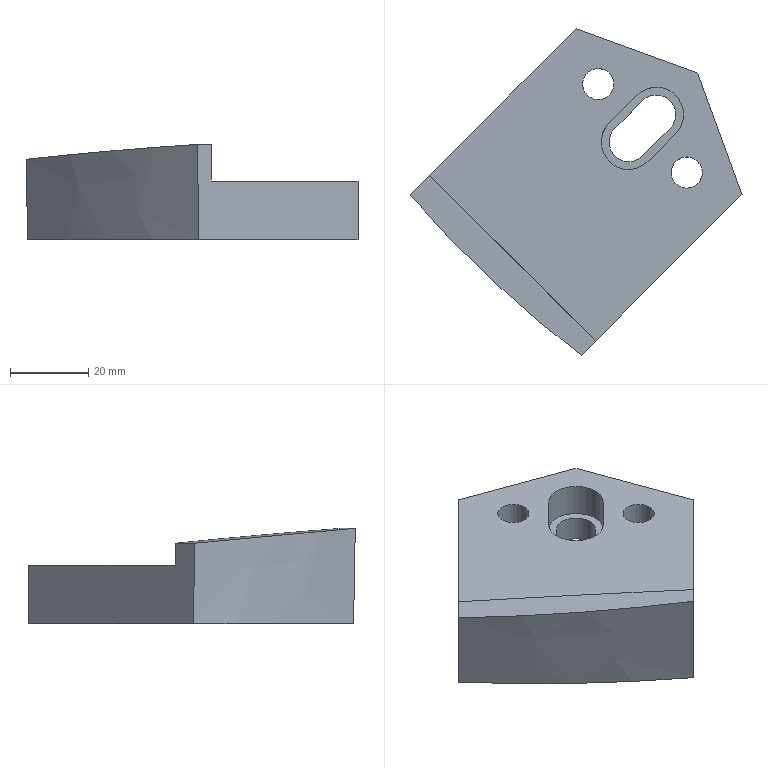Part | NX | features solid 2 | 1 solid | 20 faces | box 84.947 x 83.544 x 24.376 mm | volume 58100 mm3 | plane 12 | cylinder 6 | spline 2 | commonest cylinder face diameters 8 x2 10 x2 14 x2
STEP:
#1=CARTESIAN_POINT('',(-1044.923,370.,-23.5));
#2=VERTEX_POINT('',#1);
#3=CARTESIAN_POINT('',(-1044.923,370.,-30.));
#4=VERTEX_POINT('',#3);
#5=CARTESIAN_POINT('',(-1044.923,370.,-5.));
#6=DIRECTION('',(0.,0.,-1.));
#7=VECTOR('',#6,1000.);
#8=LINE('',#5,#7);
#9=EDGE_CURVE('',#2,#4,#8,.T.);
#10=ORIENTED_EDGE('',*,*,#9,.F.);
#11=CARTESIAN_POINT('',(-1037.852,362.929,-23.5));
#12=VERTEX_POINT('',#11);
#13=CARTESIAN_POINT('',(-1041.387,366.464,-23.5));
#14=DIRECTION('',(0.,0.,1.));
#15=DIRECTION('',(0.7071,0.7071,0.));
#16=AXIS2_PLACEMENT_3D('',#13,#14,#15);
#17=CIRCLE('',#16,5.);
#18=EDGE_CURVE('',#2,#12,#17,.T.);
#19=ORIENTED_EDGE('',*,*,#18,.T.);
#20=CARTESIAN_POINT('',(-1037.852,362.929,-30.));
#21=VERTEX_POINT('',#20);
#22=CARTESIAN_POINT('',(-1037.852,362.929,-5.));
#23=DIRECTION('',(0.,0.,-1.));
#24=VECTOR('',#23,1000.);
#25=LINE('',#22,#24);
#26=EDGE_CURVE('',#12,#21,#25,.T.);
#27=ORIENTED_EDGE('',*,*,#26,.T.);
#28=CARTESIAN_POINT('',(-1041.387,366.464,-30.));
#29=DIRECTION('',(0.,0.,1.));
#30=DIRECTION('',(0.7071,0.7071,0.));
#31=AXIS2_PLACEMENT_3D('',#28,#29,#30);
#32=CIRCLE('',#31,5.);
#33=EDGE_CURVE('',#4,#21,#32,.T.);
#34=ORIENTED_EDGE('',*,*,#33,.F.);
#35=EDGE_LOOP('',(#10,#19,#27,#34));
#36=FACE_BOUND('',#35,.T.);
#37=CARTESIAN_POINT('',(-1041.387,366.464,-5.));
#38=DIRECTION('',(0.,0.,-1.));
#39=DIRECTION('',(-0.7071,-0.7071,0.));
#40=AXIS2_PLACEMENT_3D('',#37,#38,#39);
#41=CYLINDRICAL_SURFACE('',#40,5.);
#42=ADVANCED_FACE('',(#36),#41,.F.);
#43=CARTESIAN_POINT('',(-1037.852,377.071,-23.5));
#44=VERTEX_POINT('',#43);
#45=CARTESIAN_POINT('',(-1044.923,370.,-23.5));
#46=DIRECTION('',(0.7071,0.7071,0.));
#47=VECTOR('',#46,1000.);
#48=LINE('',#45,#47);
#49=EDGE_CURVE('',#2,#44,#48,.T.);
#50=ORIENTED_EDGE('',*,*,#49,.F.);
#51=ORIENTED_EDGE('',*,*,#9,.T.);
#52=CARTESIAN_POINT('',(-1037.852,377.071,-30.));
#53=VERTEX_POINT('',#52);
#54=CARTESIAN_POINT('',(-1044.923,370.,-30.));
#55=DIRECTION('',(0.7071,0.7071,0.));
#56=VECTOR('',#55,1000.);
#57=LINE('',#54,#56);
#58=EDGE_CURVE('',#4,#53,#57,.T.);
#59=ORIENTED_EDGE('',*,*,#58,.T.);
#60=CARTESIAN_POINT('',(-1037.852,377.071,-5.));
#61=DIRECTION('',(0.,0.,-1.));
#62=VECTOR('',#61,1000.);
#63=LINE('',#60,#62);
#64=EDGE_CURVE('',#44,#53,#63,.T.);
#65=ORIENTED_EDGE('',*,*,#64,.F.);
#66=EDGE_LOOP('',(#50,#51,#59,#65));
#67=FACE_BOUND('',#66,.T.);
#68=CARTESIAN_POINT('',(-1044.923,370.,-5.));
#69=DIRECTION('',(-0.7071,0.7071,0.));
#70=DIRECTION('',(0.,0.,1.));
#71=AXIS2_PLACEMENT_3D('',#68,#69,#70);
#72=PLANE('',#71);
#73=ADVANCED_FACE('',(#67),#72,.F.);
#74=CARTESIAN_POINT('',(-1030.78,370.,-23.5));
#75=VERTEX_POINT('',#74);
#76=CARTESIAN_POINT('',(-1030.78,370.,-30.));
#77=VERTEX_POINT('',#76);
#78=CARTESIAN_POINT('',(-1030.78,370.,-5.));
#79=DIRECTION('',(0.,0.,-1.));
#80=VECTOR('',#79,1000.);
#81=LINE('',#78,#80);
#82=EDGE_CURVE('',#75,#77,#81,.T.);
#83=ORIENTED_EDGE('',*,*,#82,.F.);
#84=CARTESIAN_POINT('',(-1034.316,373.536,-23.5));
#85=DIRECTION('',(0.,0.,1.));
#86=DIRECTION('',(0.7071,0.7071,0.));
#87=AXIS2_PLACEMENT_3D('',#84,#85,#86);
#88=CIRCLE('',#87,5.);
#89=EDGE_CURVE('',#75,#44,#88,.T.);
#90=ORIENTED_EDGE('',*,*,#89,.T.);
#91=ORIENTED_EDGE('',*,*,#64,.T.);
#92=CARTESIAN_POINT('',(-1034.316,373.536,-30.));
#93=DIRECTION('',(0.,0.,1.));
#94=DIRECTION('',(0.7071,0.7071,0.));
#95=AXIS2_PLACEMENT_3D('',#92,#93,#94);
#96=CIRCLE('',#95,5.);
#97=EDGE_CURVE('',#77,#53,#96,.T.);
#98=ORIENTED_EDGE('',*,*,#97,.F.);
#99=EDGE_LOOP('',(#83,#90,#91,#98));
#100=FACE_BOUND('',#99,.T.);
#101=CARTESIAN_POINT('',(-1034.316,373.536,-5.));
#102=DIRECTION('',(0.,0.,-1.));
#103=DIRECTION('',(-0.7071,-0.7071,0.));
#104=AXIS2_PLACEMENT_3D('',#101,#102,#103);
#105=CYLINDRICAL_SURFACE('',#104,5.);
#106=ADVANCED_FACE('',(#100),#105,.F.);
#107=ORIENTED_EDGE('',*,*,#26,.F.);
#108=CARTESIAN_POINT('',(-1037.852,362.929,-23.5));
#109=DIRECTION('',(0.7071,0.7071,0.));
#110=VECTOR('',#109,1000.);
#111=LINE('',#108,#110);
#112=EDGE_CURVE('',#12,#75,#111,.T.);
#113=ORIENTED_EDGE('',*,*,#112,.T.);
#114=ORIENTED_EDGE('',*,*,#82,.T.);
#115=CARTESIAN_POINT('',(-1037.852,362.929,-30.));
#116=DIRECTION('',(0.7071,0.7071,0.));
#117=VECTOR('',#116,1000.);
#118=LINE('',#115,#117);
#119=EDGE_CURVE('',#21,#77,#118,.T.);
#120=ORIENTED_EDGE('',*,*,#119,.F.);
#121=EDGE_LOOP('',(#107,#113,#114,#120));
#122=FACE_BOUND('',#121,.T.);
#123=CARTESIAN_POINT('',(-1037.852,362.929,-5.));
#124=DIRECTION('',(-0.7071,0.7071,0.));
#125=DIRECTION('',(0.,0.,1.));
#126=AXIS2_PLACEMENT_3D('',#123,#124,#125);
#127=PLANE('',#126);
#128=ADVANCED_FACE('',(#122),#127,.T.);
#129=CARTESIAN_POINT('',(-1097.335,352.943,-9.433));
#130=VERTEX_POINT('',#129);
#131=CARTESIAN_POINT('',(-1053.506,311.919,-5.624));
#132=VERTEX_POINT('',#131);
#133=CARTESIAN_POINT('',(-1097.335,352.943,-9.433));
#134=CARTESIAN_POINT('',(-1081.965,335.2,-7.728));
#135=CARTESIAN_POINT('',(-1066.734,321.97,-6.521));
#136=CARTESIAN_POINT('',(-1053.506,311.919,-5.624));
#137=B_SPLINE_CURVE_WITH_KNOTS('',3,(#133,#134,#135,#136),.UNSPECIFIED.,.F.,.F.,(4,4),(0.,1.),.UNSPECIFIED.);
#138=EDGE_CURVE('',#130,#132,#137,.T.);
#139=ORIENTED_EDGE('',*,*,#138,.F.);
#140=CARTESIAN_POINT('',(-1096.905,353.373,-30.));
#141=VERTEX_POINT('',#140);
#142=CARTESIAN_POINT('',(-1096.905,353.373,-30.));
#143=CARTESIAN_POINT('',(-1097.048,353.23,-23.144));
#144=CARTESIAN_POINT('',(-1097.192,353.086,-16.288));
#145=CARTESIAN_POINT('',(-1097.335,352.943,-9.433));
#146=B_SPLINE_CURVE_WITH_KNOTS('',3,(#142,#143,#144,#145),.UNSPECIFIED.,.F.,.F.,(4,4),(0.,1.),.UNSPECIFIED.);
#147=EDGE_CURVE('',#130,#141,#146,.F.);
#148=ORIENTED_EDGE('',*,*,#147,.T.);
#149=CARTESIAN_POINT('',(-1053.079,312.347,-30.));
#150=VERTEX_POINT('',#149);
#151=CARTESIAN_POINT('',(-1053.079,312.347,-30.));
#152=CARTESIAN_POINT('',(-1069.242,324.631,-30.));
#153=CARTESIAN_POINT('',(-1083.851,338.306,-30.));
#154=CARTESIAN_POINT('',(-1096.905,353.373,-30.));
#155=B_SPLINE_CURVE_WITH_KNOTS('',3,(#151,#152,#153,#154),.UNSPECIFIED.,.F.,.F.,(4,4),(0.,1.),.UNSPECIFIED.);
#156=EDGE_CURVE('',#150,#141,#155,.T.);
#157=ORIENTED_EDGE('',*,*,#156,.F.);
#158=CARTESIAN_POINT('',(-1053.506,311.919,-5.624));
#159=CARTESIAN_POINT('',(-1053.364,312.062,-13.749));
#160=CARTESIAN_POINT('',(-1053.221,312.204,-21.875));
#161=CARTESIAN_POINT('',(-1053.079,312.347,-30.));
#162=B_SPLINE_CURVE_WITH_KNOTS('',3,(#158,#159,#160,#161),.UNSPECIFIED.,.F.,.F.,(4,4),(0.,1.),.UNSPECIFIED.);
#163=EDGE_CURVE('',#132,#150,#162,.T.);
#164=ORIENTED_EDGE('',*,*,#163,.F.);
#165=EDGE_LOOP('',(#139,#148,#157,#164));
#166=FACE_BOUND('',#165,.T.);
#167=CARTESIAN_POINT('',(-1097.964,353.666,-9.385));
#168=CARTESIAN_POINT('',(-1097.598,353.658,-18.565));
#169=CARTESIAN_POINT('',(-1097.232,353.65,-27.744));
#170=CARTESIAN_POINT('',(-1096.866,353.641,-36.924));
#171=CARTESIAN_POINT('',(-1084.633,338.147,-6.904));
#172=CARTESIAN_POINT('',(-1084.289,338.165,-16.095));
#173=CARTESIAN_POINT('',(-1083.946,338.184,-25.286));
#174=CARTESIAN_POINT('',(-1083.602,338.202,-34.477));
#175=CARTESIAN_POINT('',(-1069.75,324.15,-4.59));
#176=CARTESIAN_POINT('',(-1069.43,324.192,-13.792));
#177=CARTESIAN_POINT('',(-1069.111,324.234,-22.994));
#178=CARTESIAN_POINT('',(-1068.792,324.275,-32.196));
#179=CARTESIAN_POINT('',(-1053.315,311.676,-2.442));
#180=CARTESIAN_POINT('',(-1053.022,311.738,-11.655));
#181=CARTESIAN_POINT('',(-1052.729,311.8,-20.868));
#182=CARTESIAN_POINT('',(-1052.436,311.862,-30.081));
#183=B_SPLINE_SURFACE_WITH_KNOTS('',3,3,((#167,#168,#169,#170),(#171,#172,#173,#174),(#175,#176,#177,#178),(#179,#180,#181,#182)),.UNSPECIFIED.,.F.,.F.,.F.,(4,4),(4,4),(0.008791,0.2308),(4.372,5.616),.UNSPECIFIED.);
#184=ADVANCED_FACE('',(#166),#183,.F.);
#185=CARTESIAN_POINT('',(-1049.872,315.553,-5.624));
#186=VERTEX_POINT('',#185);
#187=CARTESIAN_POINT('',(-1049.872,315.553,-15.));
#188=VERTEX_POINT('',#187);
#189=CARTESIAN_POINT('',(-1049.872,315.553,-5.));
#190=DIRECTION('',(0.,0.,-1.));
#191=VECTOR('',#190,1000.);
#192=LINE('',#189,#191);
#193=EDGE_CURVE('',#186,#188,#192,.T.);
#194=ORIENTED_EDGE('',*,*,#193,.F.);
#195=CARTESIAN_POINT('',(-1052.348,313.077,-5.624));
#196=DIRECTION('',(-0.7071,-0.7071,0.));
#197=VECTOR('',#196,1000.);
#198=LINE('',#195,#197);
#199=EDGE_CURVE('',#186,#132,#198,.T.);
#200=ORIENTED_EDGE('',*,*,#199,.T.);
#201=ORIENTED_EDGE('',*,*,#163,.T.);
#202=CARTESIAN_POINT('',(-1012.388,353.037,-30.));
#203=VERTEX_POINT('',#202);
#204=CARTESIAN_POINT('',(-1055.529,309.896,-30.));
#205=DIRECTION('',(0.7071,0.7071,0.));
#206=VECTOR('',#205,1000.);
#207=LINE('',#204,#206);
#208=EDGE_CURVE('',#150,#203,#207,.T.);
#209=ORIENTED_EDGE('',*,*,#208,.T.);
#210=CARTESIAN_POINT('',(-1012.388,353.037,-15.));
#211=VERTEX_POINT('',#210);
#212=CARTESIAN_POINT('',(-1012.388,353.037,-5.));
#213=DIRECTION('',(0.,0.,-1.));
#214=VECTOR('',#213,1000.);
#215=LINE('',#212,#214);
#216=EDGE_CURVE('',#211,#203,#215,.T.);
#217=ORIENTED_EDGE('',*,*,#216,.F.);
#218=CARTESIAN_POINT('',(-1055.529,309.896,-15.));
#219=DIRECTION('',(0.7071,0.7071,0.));
#220=VECTOR('',#219,1000.);
#221=LINE('',#218,#220);
#222=EDGE_CURVE('',#188,#211,#221,.T.);
#223=ORIENTED_EDGE('',*,*,#222,.F.);
#224=EDGE_LOOP('',(#194,#200,#201,#209,#217,#223));
#225=FACE_BOUND('',#224,.T.);
#226=CARTESIAN_POINT('',(-1055.529,309.896,-5.));
#227=DIRECTION('',(-0.7071,0.7071,0.));
#228=DIRECTION('',(-0.7071,-0.7071,0.));
#229=AXIS2_PLACEMENT_3D('',#226,#227,#228);
#230=PLANE('',#229);
#231=ADVANCED_FACE('',(#225),#230,.F.);
#232=CARTESIAN_POINT('',(-1023.709,384.142,-15.));
#233=VERTEX_POINT('',#232);
#234=CARTESIAN_POINT('',(-1012.388,353.037,-15.));
#235=DIRECTION('',(-0.342,0.9397,0.));
#236=VECTOR('',#235,1000.);
#237=LINE('',#234,#236);
#238=EDGE_CURVE('',#211,#233,#237,.T.);
#239=ORIENTED_EDGE('',*,*,#238,.F.);
#240=ORIENTED_EDGE('',*,*,#216,.T.);
#241=CARTESIAN_POINT('',(-1023.709,384.142,-30.));
#242=VERTEX_POINT('',#241);
#243=CARTESIAN_POINT('',(-1012.388,353.037,-30.));
#244=DIRECTION('',(-0.342,0.9397,0.));
#245=VECTOR('',#244,1000.);
#246=LINE('',#243,#245);
#247=EDGE_CURVE('',#203,#242,#246,.T.);
#248=ORIENTED_EDGE('',*,*,#247,.T.);
#249=CARTESIAN_POINT('',(-1023.709,384.142,-5.));
#250=DIRECTION('',(0.,0.,-1.));
#251=VECTOR('',#250,1000.);
#252=LINE('',#249,#251);
#253=EDGE_CURVE('',#233,#242,#252,.T.);
#254=ORIENTED_EDGE('',*,*,#253,.F.);
#255=EDGE_LOOP('',(#239,#240,#248,#254));
#256=FACE_BOUND('',#255,.T.);
#257=CARTESIAN_POINT('',(-1012.388,353.037,-5.));
#258=DIRECTION('',(-0.9397,-0.342,0.));
#259=DIRECTION('',(0.342,-0.9397,0.));
#260=AXIS2_PLACEMENT_3D('',#257,#258,#259);
#261=PLANE('',#260);
#262=ADVANCED_FACE('',(#256),#261,.F.);
#263=CARTESIAN_POINT('',(-1054.814,395.463,-15.));
#264=VERTEX_POINT('',#263);
#265=CARTESIAN_POINT('',(-1054.814,395.463,-30.));
#266=VERTEX_POINT('',#265);
#267=CARTESIAN_POINT('',(-1054.814,395.463,-5.));
#268=DIRECTION('',(0.,0.,-1.));
#269=VECTOR('',#268,1000.);
#270=LINE('',#267,#269);
#271=EDGE_CURVE('',#264,#266,#270,.T.);
#272=ORIENTED_EDGE('',*,*,#271,.F.);
#273=CARTESIAN_POINT('',(-1054.814,395.463,-15.));
#274=DIRECTION('',(0.9397,-0.342,0.));
#275=VECTOR('',#274,1000.);
#276=LINE('',#273,#275);
#277=EDGE_CURVE('',#264,#233,#276,.T.);
#278=ORIENTED_EDGE('',*,*,#277,.T.);
#279=ORIENTED_EDGE('',*,*,#253,.T.);
#280=CARTESIAN_POINT('',(-1054.814,395.463,-30.));
#281=DIRECTION('',(0.9397,-0.342,0.));
#282=VECTOR('',#281,1000.);
#283=LINE('',#280,#282);
#284=EDGE_CURVE('',#266,#242,#283,.T.);
#285=ORIENTED_EDGE('',*,*,#284,.F.);
#286=EDGE_LOOP('',(#272,#278,#279,#285));
#287=FACE_BOUND('',#286,.T.);
#288=CARTESIAN_POINT('',(-1054.814,395.463,-5.));
#289=DIRECTION('',(0.342,0.9397,0.));
#290=DIRECTION('',(-0.9397,0.342,0.));
#291=AXIS2_PLACEMENT_3D('',#288,#289,#290);
#292=PLANE('',#291);
#293=ADVANCED_FACE('',(#287),#292,.T.);
#294=CARTESIAN_POINT('',(-1046.337,384.142,-15.));
#295=VERTEX_POINT('',#294);
#296=CARTESIAN_POINT('',(-1049.165,381.314,-15.));
#297=DIRECTION('',(0.,0.,1.));
#298=DIRECTION('',(0.7071,0.7071,0.));
#299=AXIS2_PLACEMENT_3D('',#296,#297,#298);
#300=CIRCLE('',#299,4.);
#301=EDGE_CURVE('',#295,#295,#300,.T.);
#302=ORIENTED_EDGE('',*,*,#301,.T.);
#303=EDGE_LOOP('',(#302));
#304=FACE_BOUND('',#303,.T.);
#305=CARTESIAN_POINT('',(-1046.337,384.142,-30.));
#306=VERTEX_POINT('',#305);
#307=CARTESIAN_POINT('',(-1049.165,381.314,-30.));
#308=DIRECTION('',(0.,0.,1.));
#309=DIRECTION('',(0.7071,0.7071,0.));
#310=AXIS2_PLACEMENT_3D('',#307,#308,#309);
#311=CIRCLE('',#310,4.);
#312=EDGE_CURVE('',#306,#306,#311,.T.);
#313=ORIENTED_EDGE('',*,*,#312,.F.);
#314=EDGE_LOOP('',(#313));
#315=FACE_BOUND('',#314,.T.);
#316=CARTESIAN_POINT('',(-1049.165,381.314,-5.));
#317=DIRECTION('',(0.,0.,-1.));
#318=DIRECTION('',(-0.7071,-0.7071,0.));
#319=AXIS2_PLACEMENT_3D('',#316,#317,#318);
#320=CYLINDRICAL_SURFACE('',#319,4.);
#321=ADVANCED_FACE('',(#304,#315),#320,.F.);
#322=CARTESIAN_POINT('',(-1092.299,357.979,-9.433));
#323=VERTEX_POINT('',#322);
#324=CARTESIAN_POINT('',(-1094.775,355.503,-9.433));
#325=DIRECTION('',(-0.7071,-0.7071,0.));
#326=VECTOR('',#325,1000.);
#327=LINE('',#324,#326);
#328=EDGE_CURVE('',#323,#130,#327,.T.);
#329=ORIENTED_EDGE('',*,*,#328,.F.);
#330=CARTESIAN_POINT('',(-1092.299,357.979,-15.));
#331=VERTEX_POINT('',#330);
#332=CARTESIAN_POINT('',(-1092.299,357.979,-5.));
#333=DIRECTION('',(0.,0.,-1.));
#334=VECTOR('',#333,1000.);
#335=LINE('',#332,#334);
#336=EDGE_CURVE('',#323,#331,#335,.T.);
#337=ORIENTED_EDGE('',*,*,#336,.T.);
#338=CARTESIAN_POINT('',(-1097.956,352.322,-15.));
#339=DIRECTION('',(0.7071,0.7071,0.));
#340=VECTOR('',#339,1000.);
#341=LINE('',#338,#340);
#342=EDGE_CURVE('',#331,#264,#341,.T.);
#343=ORIENTED_EDGE('',*,*,#342,.T.);
#344=ORIENTED_EDGE('',*,*,#271,.T.);
#345=CARTESIAN_POINT('',(-1097.956,352.322,-30.));
#346=DIRECTION('',(0.7071,0.7071,0.));
#347=VECTOR('',#346,1000.);
#348=LINE('',#345,#347);
#349=EDGE_CURVE('',#141,#266,#348,.T.);
#350=ORIENTED_EDGE('',*,*,#349,.F.);
#351=ORIENTED_EDGE('',*,*,#147,.F.);
#352=EDGE_LOOP('',(#329,#337,#343,#344,#350,#351));
#353=FACE_BOUND('',#352,.T.);
#354=CARTESIAN_POINT('',(-1097.956,352.322,-5.));
#355=DIRECTION('',(-0.7071,0.7071,0.));
#356=DIRECTION('',(-0.7071,-0.7071,0.));
#357=AXIS2_PLACEMENT_3D('',#354,#355,#356);
#358=PLANE('',#357);
#359=ADVANCED_FACE('',(#353),#358,.T.);
#360=CARTESIAN_POINT('',(-1023.709,361.515,-15.));
#361=VERTEX_POINT('',#360);
#362=CARTESIAN_POINT('',(-1026.538,358.686,-15.));
#363=DIRECTION('',(0.,0.,1.));
#364=DIRECTION('',(0.7071,0.7071,0.));
#365=AXIS2_PLACEMENT_3D('',#362,#363,#364);
#366=CIRCLE('',#365,4.);
#367=EDGE_CURVE('',#361,#361,#366,.F.);
#368=ORIENTED_EDGE('',*,*,#367,.F.);
#369=EDGE_LOOP('',(#368));
#370=FACE_BOUND('',#369,.T.);
#371=CARTESIAN_POINT('',(-1023.709,361.515,-30.));
#372=VERTEX_POINT('',#371);
#373=CARTESIAN_POINT('',(-1026.538,358.686,-30.));
#374=DIRECTION('',(0.,0.,-1.));
#375=DIRECTION('',(0.7071,0.7071,0.));
#376=AXIS2_PLACEMENT_3D('',#373,#374,#375);
#377=CIRCLE('',#376,4.);
#378=EDGE_CURVE('',#372,#372,#377,.T.);
#379=ORIENTED_EDGE('',*,*,#378,.T.);
#380=EDGE_LOOP('',(#379));
#381=FACE_BOUND('',#380,.T.);
#382=CARTESIAN_POINT('',(-1026.538,358.686,-5.));
#383=DIRECTION('',(0.,0.,-1.));
#384=DIRECTION('',(-0.7071,-0.7071,0.));
#385=AXIS2_PLACEMENT_3D('',#382,#383,#384);
#386=CYLINDRICAL_SURFACE('',#385,4.);
#387=ADVANCED_FACE('',(#370,#381),#386,.F.);
#388=ORIENTED_EDGE('',*,*,#33,.T.);
#389=ORIENTED_EDGE('',*,*,#119,.T.);
#390=ORIENTED_EDGE('',*,*,#97,.T.);
#391=ORIENTED_EDGE('',*,*,#58,.F.);
#392=EDGE_LOOP('',(#388,#389,#390,#391));
#393=FACE_BOUND('',#392,.T.);
#394=ORIENTED_EDGE('',*,*,#156,.T.);
#395=ORIENTED_EDGE('',*,*,#349,.T.);
#396=ORIENTED_EDGE('',*,*,#284,.T.);
#397=ORIENTED_EDGE('',*,*,#247,.F.);
#398=ORIENTED_EDGE('',*,*,#208,.F.);
#399=EDGE_LOOP('',(#394,#395,#396,#397,#398));
#400=FACE_BOUND('',#399,.T.);
#401=ORIENTED_EDGE('',*,*,#312,.T.);
#402=EDGE_LOOP('',(#401));
#403=FACE_BOUND('',#402,.T.);
#404=ORIENTED_EDGE('',*,*,#378,.F.);
#405=EDGE_LOOP('',(#404));
#406=FACE_BOUND('',#405,.T.);
#407=CARTESIAN_POINT('',(-1097.956,352.322,-30.));
#408=DIRECTION('',(0.,0.,1.));
#409=DIRECTION('',(0.7071,0.7071,0.));
#410=AXIS2_PLACEMENT_3D('',#407,#408,#409);
#411=PLANE('',#410);
#412=ADVANCED_FACE('',(#393,#400,#403,#406),#411,.F.);
#413=CARTESIAN_POINT('',(-1046.337,371.414,-15.));
#414=VERTEX_POINT('',#413);
#415=CARTESIAN_POINT('',(-1039.266,378.485,-15.));
#416=VERTEX_POINT('',#415);
#417=CARTESIAN_POINT('',(-1046.337,371.414,-15.));
#418=DIRECTION('',(0.7071,0.7071,0.));
#419=VECTOR('',#418,1000.);
#420=LINE('',#417,#419);
#421=EDGE_CURVE('',#414,#416,#420,.T.);
#422=ORIENTED_EDGE('',*,*,#421,.F.);
#423=CARTESIAN_POINT('',(-1046.337,371.414,-23.5));
#424=VERTEX_POINT('',#423);
#425=CARTESIAN_POINT('',(-1046.337,371.414,0.));
#426=DIRECTION('',(0.,0.,-1.));
#427=VECTOR('',#426,1000.);
#428=LINE('',#425,#427);
#429=EDGE_CURVE('',#414,#424,#428,.T.);
#430=ORIENTED_EDGE('',*,*,#429,.T.);
#431=CARTESIAN_POINT('',(-1039.266,378.485,-23.5));
#432=VERTEX_POINT('',#431);
#433=CARTESIAN_POINT('',(-1046.337,371.414,-23.5));
#434=DIRECTION('',(0.7071,0.7071,0.));
#435=VECTOR('',#434,1000.);
#436=LINE('',#433,#435);
#437=EDGE_CURVE('',#424,#432,#436,.T.);
#438=ORIENTED_EDGE('',*,*,#437,.T.);
#439=CARTESIAN_POINT('',(-1039.266,378.485,0.));
#440=DIRECTION('',(0.,0.,-1.));
#441=VECTOR('',#440,1000.);
#442=LINE('',#439,#441);
#443=EDGE_CURVE('',#416,#432,#442,.T.);
#444=ORIENTED_EDGE('',*,*,#443,.F.);
#445=EDGE_LOOP('',(#422,#430,#438,#444));
#446=FACE_BOUND('',#445,.T.);
#447=CARTESIAN_POINT('',(-1046.337,371.414,0.));
#448=DIRECTION('',(-0.7071,0.7071,0.));
#449=DIRECTION('',(0.,0.,1.));
#450=AXIS2_PLACEMENT_3D('',#447,#448,#449);
#451=PLANE('',#450);
#452=ADVANCED_FACE('',(#446),#451,.F.);
#453=CARTESIAN_POINT('',(-1029.366,368.586,-15.));
#454=VERTEX_POINT('',#453);
#455=CARTESIAN_POINT('',(-1034.316,373.536,-15.));
#456=DIRECTION('',(0.,0.,1.));
#457=DIRECTION('',(0.7071,0.7071,0.));
#458=AXIS2_PLACEMENT_3D('',#455,#456,#457);
#459=CIRCLE('',#458,7.);
#460=EDGE_CURVE('',#416,#454,#459,.F.);
#461=ORIENTED_EDGE('',*,*,#460,.F.);
#462=ORIENTED_EDGE('',*,*,#443,.T.);
#463=CARTESIAN_POINT('',(-1029.366,368.586,-23.5));
#464=VERTEX_POINT('',#463);
#465=CARTESIAN_POINT('',(-1034.316,373.536,-23.5));
#466=DIRECTION('',(0.,0.,-1.));
#467=DIRECTION('',(0.7071,0.7071,0.));
#468=AXIS2_PLACEMENT_3D('',#465,#466,#467);
#469=CIRCLE('',#468,7.);
#470=EDGE_CURVE('',#432,#464,#469,.T.);
#471=ORIENTED_EDGE('',*,*,#470,.T.);
#472=CARTESIAN_POINT('',(-1029.366,368.586,0.));
#473=DIRECTION('',(0.,0.,-1.));
#474=VECTOR('',#473,1000.);
#475=LINE('',#472,#474);
#476=EDGE_CURVE('',#454,#464,#475,.T.);
#477=ORIENTED_EDGE('',*,*,#476,.F.);
#478=EDGE_LOOP('',(#461,#462,#471,#477));
#479=FACE_BOUND('',#478,.T.);
#480=CARTESIAN_POINT('',(-1034.316,373.536,0.));
#481=DIRECTION('',(0.,0.,-1.));
#482=DIRECTION('',(-0.7071,-0.7071,0.));
#483=AXIS2_PLACEMENT_3D('',#480,#481,#482);
#484=CYLINDRICAL_SURFACE('',#483,7.);
#485=ADVANCED_FACE('',(#479),#484,.F.);
#486=CARTESIAN_POINT('',(-1036.437,361.515,-15.));
#487=VERTEX_POINT('',#486);
#488=CARTESIAN_POINT('',(-1036.437,361.515,-23.5));
#489=VERTEX_POINT('',#488);
#490=CARTESIAN_POINT('',(-1036.437,361.515,0.));
#491=DIRECTION('',(0.,0.,-1.));
#492=VECTOR('',#491,1000.);
#493=LINE('',#490,#492);
#494=EDGE_CURVE('',#487,#489,#493,.T.);
#495=ORIENTED_EDGE('',*,*,#494,.F.);
#496=CARTESIAN_POINT('',(-1036.437,361.515,-15.));
#497=DIRECTION('',(0.7071,0.7071,0.));
#498=VECTOR('',#497,1000.);
#499=LINE('',#496,#498);
#500=EDGE_CURVE('',#487,#454,#499,.T.);
#501=ORIENTED_EDGE('',*,*,#500,.T.);
#502=ORIENTED_EDGE('',*,*,#476,.T.);
#503=CARTESIAN_POINT('',(-1036.437,361.515,-23.5));
#504=DIRECTION('',(0.7071,0.7071,0.));
#505=VECTOR('',#504,1000.);
#506=LINE('',#503,#505);
#507=EDGE_CURVE('',#489,#464,#506,.T.);
#508=ORIENTED_EDGE('',*,*,#507,.F.);
#509=EDGE_LOOP('',(#495,#501,#502,#508));
#510=FACE_BOUND('',#509,.T.);
#511=CARTESIAN_POINT('',(-1036.437,361.515,0.));
#512=DIRECTION('',(-0.7071,0.7071,0.));
#513=DIRECTION('',(0.,0.,1.));
#514=AXIS2_PLACEMENT_3D('',#511,#512,#513);
#515=PLANE('',#514);
#516=ADVANCED_FACE('',(#510),#515,.T.);
#517=ORIENTED_EDGE('',*,*,#429,.F.);
#518=CARTESIAN_POINT('',(-1041.387,366.464,-15.));
#519=DIRECTION('',(0.,0.,1.));
#520=DIRECTION('',(0.7071,0.7071,0.));
#521=AXIS2_PLACEMENT_3D('',#518,#519,#520);
#522=CIRCLE('',#521,7.);
#523=EDGE_CURVE('',#414,#487,#522,.T.);
#524=ORIENTED_EDGE('',*,*,#523,.T.);
#525=ORIENTED_EDGE('',*,*,#494,.T.);
#526=CARTESIAN_POINT('',(-1041.387,366.464,-23.5));
#527=DIRECTION('',(0.,0.,1.));
#528=DIRECTION('',(0.7071,0.7071,0.));
#529=AXIS2_PLACEMENT_3D('',#526,#527,#528);
#530=CIRCLE('',#529,7.);
#531=EDGE_CURVE('',#424,#489,#530,.T.);
#532=ORIENTED_EDGE('',*,*,#531,.F.);
#533=EDGE_LOOP('',(#517,#524,#525,#532));
#534=FACE_BOUND('',#533,.T.);
#535=CARTESIAN_POINT('',(-1041.387,366.464,0.));
#536=DIRECTION('',(0.,0.,-1.));
#537=DIRECTION('',(-0.7071,-0.7071,0.));
#538=AXIS2_PLACEMENT_3D('',#535,#536,#537);
#539=CYLINDRICAL_SURFACE('',#538,7.);
#540=ADVANCED_FACE('',(#534),#539,.F.);
#541=ORIENTED_EDGE('',*,*,#49,.T.);
#542=ORIENTED_EDGE('',*,*,#89,.F.);
#543=ORIENTED_EDGE('',*,*,#112,.F.);
#544=ORIENTED_EDGE('',*,*,#18,.F.);
#545=EDGE_LOOP('',(#541,#542,#543,#544));
#546=FACE_BOUND('',#545,.T.);
#547=ORIENTED_EDGE('',*,*,#437,.F.);
#548=ORIENTED_EDGE('',*,*,#531,.T.);
#549=ORIENTED_EDGE('',*,*,#507,.T.);
#550=ORIENTED_EDGE('',*,*,#470,.F.);
#551=EDGE_LOOP('',(#547,#548,#549,#550));
#552=FACE_BOUND('',#551,.T.);
#553=CARTESIAN_POINT('',(-1034.316,373.536,-23.5));
#554=DIRECTION('',(0.,0.,1.));
#555=DIRECTION('',(0.7071,0.7071,0.));
#556=AXIS2_PLACEMENT_3D('',#553,#554,#555);
#557=PLANE('',#556);
#558=ADVANCED_FACE('',(#546,#552),#557,.T.);
#559=CARTESIAN_POINT('',(-1049.872,315.553,-5.624));
#560=CARTESIAN_POINT('',(-1064.023,329.703,-6.715));
#561=CARTESIAN_POINT('',(-1078.165,343.845,-7.977));
#562=CARTESIAN_POINT('',(-1092.299,357.979,-9.433));
#563=B_SPLINE_CURVE_WITH_KNOTS('',3,(#559,#560,#561,#562),.UNSPECIFIED.,.F.,.F.,(4,4),(0.,0.06012),.UNSPECIFIED.);
#564=EDGE_CURVE('',#186,#323,#563,.T.);
#565=ORIENTED_EDGE('',*,*,#564,.F.);
#566=ORIENTED_EDGE('',*,*,#193,.T.);
#567=CARTESIAN_POINT('',(-1000.375,266.055,-15.));
#568=DIRECTION('',(-0.7071,0.7071,0.));
#569=VECTOR('',#568,1000.);
#570=LINE('',#567,#569);
#571=EDGE_CURVE('',#188,#331,#570,.T.);
#572=ORIENTED_EDGE('',*,*,#571,.T.);
#573=ORIENTED_EDGE('',*,*,#336,.F.);
#574=EDGE_LOOP('',(#565,#566,#572,#573));
#575=FACE_BOUND('',#574,.T.);
#576=CARTESIAN_POINT('',(-1000.375,266.055,-5.));
#577=DIRECTION('',(0.7071,0.7071,0.));
#578=DIRECTION('',(0.,0.,-1.));
#579=AXIS2_PLACEMENT_3D('',#576,#577,#578);
#580=PLANE('',#579);
#581=ADVANCED_FACE('',(#575),#580,.T.);
#582=ORIENTED_EDGE('',*,*,#301,.F.);
#583=EDGE_LOOP('',(#582));
#584=FACE_BOUND('',#583,.T.);
#585=ORIENTED_EDGE('',*,*,#367,.T.);
#586=EDGE_LOOP('',(#585));
#587=FACE_BOUND('',#586,.T.);
#588=ORIENTED_EDGE('',*,*,#523,.F.);
#589=ORIENTED_EDGE('',*,*,#421,.T.);
#590=ORIENTED_EDGE('',*,*,#460,.T.);
#591=ORIENTED_EDGE('',*,*,#500,.F.);
#592=EDGE_LOOP('',(#588,#589,#590,#591));
#593=FACE_BOUND('',#592,.T.);
#594=ORIENTED_EDGE('',*,*,#571,.F.);
#595=ORIENTED_EDGE('',*,*,#222,.T.);
#596=ORIENTED_EDGE('',*,*,#238,.T.);
#597=ORIENTED_EDGE('',*,*,#277,.F.);
#598=ORIENTED_EDGE('',*,*,#342,.F.);
#599=EDGE_LOOP('',(#594,#595,#596,#597,#598));
#600=FACE_BOUND('',#599,.T.);
#601=CARTESIAN_POINT('',(-1000.375,266.055,-15.));
#602=DIRECTION('',(0.,0.,1.));
#603=DIRECTION('',(0.7071,0.7071,0.));
#604=AXIS2_PLACEMENT_3D('',#601,#602,#603);
#605=PLANE('',#604);
#606=ADVANCED_FACE('',(#584,#587,#593,#600),#605,.T.);
#607=ORIENTED_EDGE('',*,*,#138,.T.);
#608=ORIENTED_EDGE('',*,*,#199,.F.);
#609=ORIENTED_EDGE('',*,*,#564,.T.);
#610=ORIENTED_EDGE('',*,*,#328,.T.);
#611=EDGE_LOOP('',(#607,#608,#609,#610));
#612=FACE_BOUND('',#611,.T.);
#613=CARTESIAN_POINT('',(-1048.57,316.855,-5.624));
#614=CARTESIAN_POINT('',(-1054.582,310.843,-5.624));
#615=CARTESIAN_POINT('',(-1064.119,329.506,-6.711));
#616=CARTESIAN_POINT('',(-1070.131,323.494,-6.711));
#617=CARTESIAN_POINT('',(-1078.529,343.556,-7.981));
#618=CARTESIAN_POINT('',(-1084.541,337.544,-7.981));
#619=CARTESIAN_POINT('',(-1091.358,358.919,-9.433));
#620=CARTESIAN_POINT('',(-1097.371,352.907,-9.433));
#621=B_SPLINE_SURFACE_WITH_KNOTS('',3,1,((#613,#614),(#615,#616),(#617,#618),(#619,#620)),.SURF_OF_LINEAR_EXTRUSION.,.F.,.F.,.F.,(4,4),(2,2),(0.05486,0.2386),(0.,1.),.PIECEWISE_BEZIER_KNOTS.);
#622=ADVANCED_FACE('',(#612),#621,.T.);
#623=CLOSED_SHELL('',(#42,#73,#106,#128,#184,#231,#262,#293,#321,#359,#387,#412,#452,#485,#516,#540,#558,#581,#606,#622));
#624=MANIFOLD_SOLID_BREP('',#623);
#625=(LENGTH_UNIT()NAMED_UNIT(*)SI_UNIT(.MILLI.,.METRE.));
#626=UNCERTAINTY_MEASURE_WITH_UNIT(LENGTH_MEASURE(0.0508),#625,'','');
#627=(NAMED_UNIT(*)PLANE_ANGLE_UNIT()SI_UNIT($,.RADIAN.));
#628=(NAMED_UNIT(*)SI_UNIT($,.STERADIAN.)SOLID_ANGLE_UNIT());
#629=(GEOMETRIC_REPRESENTATION_CONTEXT(3)GLOBAL_UNCERTAINTY_ASSIGNED_CONTEXT((#626))GLOBAL_UNIT_ASSIGNED_CONTEXT((#625,#627,#628))REPRESENTATION_CONTEXT('',''));
#630=ADVANCED_BREP_SHAPE_REPRESENTATION('',(#624),#629);